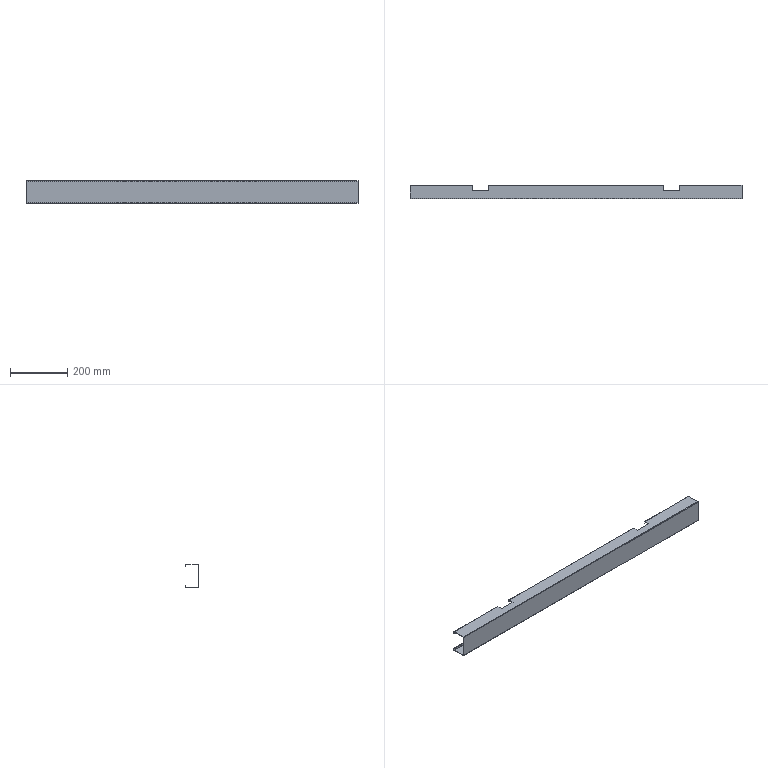Part | 1 solid | 86 faces | box 1159 x 48 x 80 mm | volume 311759 mm3 | plane 70 | cylinder 16 | commonest cylinder face diameters 0.4 x8 3.4 x8